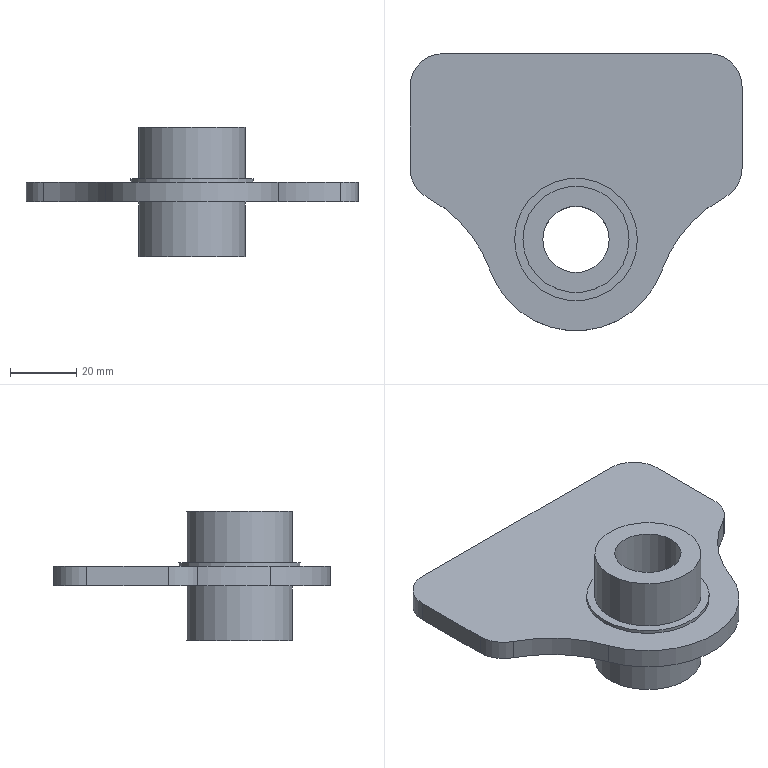CAM job | NX | 3-axis milling, drilling | part box 100 x 83.5 x 39 mm
Tools:
number,name,description,diameter,corner_radius,flute_length,length,flutes
1,D16-48-D16-100-3T-FINISH,D16-48-D16-100-3T,16.0,0.0,48.0,100.0,3
0,倒角D6-90度,倒角D6-90度,6.0,0.0,5.0,50.0,2
0,D25,Milling Tool-5 Parameters,20.0,0.0,30.0,30.0,4
Operations:
program,operation,operation_type,tool,method,geometry_group,spindle_rpm,surface_speed,feed_per_tooth,feed_cut,feed_plunge,cut_length_mm,path_length_mm,cut_time_min,machine_time_min
A1,ADAPTIVE_MILLING,CavityMilling,D16-48-D16-100-3T-FINISH,METHOD,WORKPIECE_54,3000.0,150.0,0.2222,2000.0,100.0,1869.963,1923.663,0.935,0.9404
A1,PLANAR_MILL_1_COPY,PlanarMilling,D16-48-D16-100-3T-FINISH,METHOD,A-G54,3000.0,150.0,0.1111,1000.0,100.0,934.453,1019.253,0.9345,0.9429
A1,PLANAR_MILL,PlanarMilling,D16-48-D16-100-3T-FINISH,METHOD,A-G54,3000.0,150.0,0.1111,1000.0,100.0,131.268,185.268,0.1313,0.1367
A1,FLOOR_WALL,VolumeBased25DMillingOperation,D16-48-D16-100-3T-FINISH,METHOD,A-G54,3000.0,150.0,0.1111,1000.0,100.0,1521.512,1825.908,1.522,1.552
A1,PLANAR_MILL_1,PlanarMilling,D16-48-D16-100-3T-FINISH,METHOD,A-G54,3000.0,150.0,0.1111,1000.0,100.0,195.524,284.524,0.1955,0.2044
A1,PLANAR_MILL_4,PlanarMilling,D16-48-D16-100-3T-FINISH,METHOD,A-G54,3000.0,150.0,0.1111,1000.0,100.0,2304.886,2401.886,2.305,2.315
A1,PLANAR_MILL_4_COPY,PlanarMilling,D16-48-D16-100-3T-FINISH,METHOD,A-G54,3000.0,150.0,0.0444,400.0,100.0,39.416,173.416,0.0985,0.1119
A1,PLANAR_MILL_2,PlanarMilling,倒角D6-90度,METHOD,WORKPIECE_54,3000.0,28.0,0.1333,800.0,100.0,46.243,138.243,0.0578,0.067
A1,PLANAR_MILL_3,PlanarMilling,倒角D6-90度,METHOD,A-G54,3000.0,56.0,0.1,600.0,100.0,121.239,181.239,0.2021,0.2081
A1,PLANAR_MILL_3_COPY,PlanarMilling,倒角D6-90度,METHOD,A-G54,3000.0,56.0,0.1,600.0,100.0,65.321,125.321,0.1089,0.1149
A1,DRILLING,Operation,D25,METHOD,A-G54,800.0,50.0,0.025,80.0,0.0,41.0,142.0,0.5125,0.5226